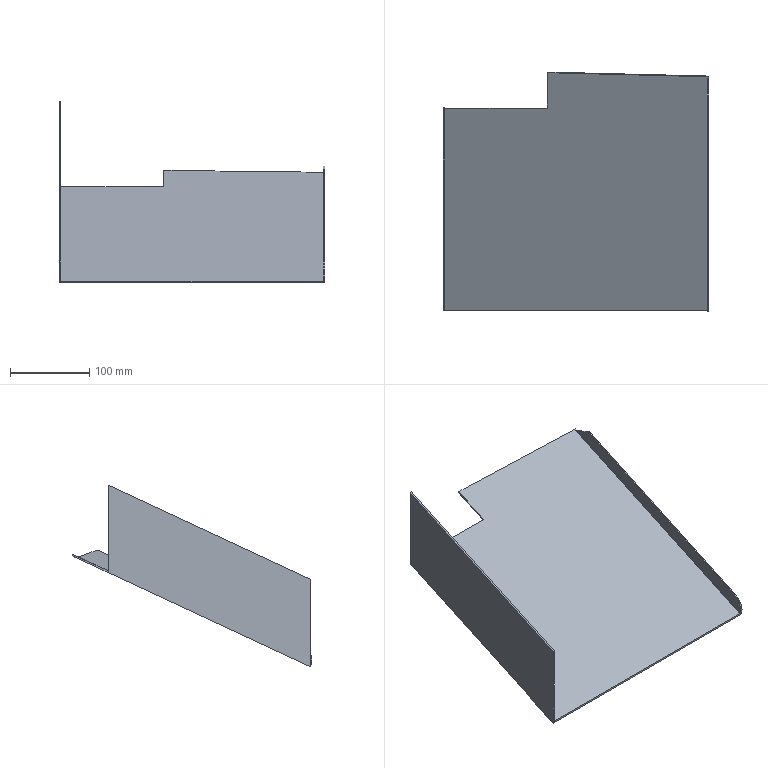Part | NX | features solid 2 | 1 solid | 15 faces | box 335 x 302.219 x 229.246 mm | volume 273833 mm3 | plane 13 | spline 1 | cylinder 1 | commonest cylinder face diameters 40 x1
STEP:
#1=CARTESIAN_POINT('',(-607.,-820.,-270.764));
#2=VERTEX_POINT('',#1);
#3=CARTESIAN_POINT('',(-938.,-820.,-270.764));
#4=VERTEX_POINT('',#3);
#5=CARTESIAN_POINT('',(1065.,-820.,-270.764));
#6=DIRECTION('',(1.,0.,0.));
#7=VECTOR('',#6,1000.);
#8=LINE('',#5,#7);
#9=EDGE_CURVE('',#2,#4,#8,.F.);
#10=ORIENTED_EDGE('',*,*,#9,.T.);
#11=CARTESIAN_POINT('',(-938.,-820.,-162.633));
#12=VERTEX_POINT('',#11);
#13=CARTESIAN_POINT('',(-938.,-820.,-730.));
#14=DIRECTION('',(0.,0.,1.));
#15=VECTOR('',#14,1000.);
#16=LINE('',#13,#15);
#17=EDGE_CURVE('',#12,#4,#16,.F.);
#18=ORIENTED_EDGE('',*,*,#17,.F.);
#19=CARTESIAN_POINT('',(-940.,-820.,-162.633));
#20=VERTEX_POINT('',#19);
#21=CARTESIAN_POINT('',(-940.,-820.,-162.633));
#22=DIRECTION('',(1.,0.,0.));
#23=VECTOR('',#22,1000.);
#24=LINE('',#21,#23);
#25=EDGE_CURVE('',#20,#12,#24,.T.);
#26=ORIENTED_EDGE('',*,*,#25,.F.);
#27=CARTESIAN_POINT('',(-940.,-820.,-272.971));
#28=VERTEX_POINT('',#27);
#29=CARTESIAN_POINT('',(-940.,-820.,-151.933));
#30=DIRECTION('',(0.,0.,1.));
#31=VECTOR('',#30,1000.);
#32=LINE('',#29,#31);
#33=EDGE_CURVE('',#28,#20,#32,.T.);
#34=ORIENTED_EDGE('',*,*,#33,.F.);
#35=CARTESIAN_POINT('',(-607.,-820.,-272.971));
#36=VERTEX_POINT('',#35);
#37=CARTESIAN_POINT('',(1065.,-820.,-272.971));
#38=DIRECTION('',(1.,0.,0.));
#39=VECTOR('',#38,1000.);
#40=LINE('',#37,#39);
#41=EDGE_CURVE('',#36,#28,#40,.F.);
#42=ORIENTED_EDGE('',*,*,#41,.F.);
#43=CARTESIAN_POINT('',(-607.,-820.,-730.));
#44=DIRECTION('',(0.,0.,1.));
#45=VECTOR('',#44,1000.);
#46=LINE('',#43,#45);
#47=EDGE_CURVE('',#2,#36,#46,.F.);
#48=ORIENTED_EDGE('',*,*,#47,.F.);
#49=EDGE_LOOP('',(#10,#18,#26,#34,#42,#48));
#50=FACE_BOUND('',#49,.T.);
#51=CARTESIAN_POINT('',(1065.,-820.,-730.));
#52=DIRECTION('',(0.,1.,0.));
#53=DIRECTION('',(-1.,0.,0.));
#54=AXIS2_PLACEMENT_3D('',#51,#52,#53);
#55=PLANE('',#54);
#56=ADVANCED_FACE('',(#50),#55,.F.);
#57=CARTESIAN_POINT('',(-808.587,-565.,-151.855));
#58=VERTEX_POINT('',#57);
#59=CARTESIAN_POINT('',(-938.,-565.,-151.855));
#60=VERTEX_POINT('',#59);
#61=CARTESIAN_POINT('',(-888.494,-565.,-151.855));
#62=DIRECTION('',(1.,0.,0.));
#63=VECTOR('',#62,1000.);
#64=LINE('',#61,#63);
#65=EDGE_CURVE('',#58,#60,#64,.F.);
#66=ORIENTED_EDGE('',*,*,#65,.T.);
#67=CARTESIAN_POINT('',(-938.,-565.167,-151.933));
#68=DIRECTION('',(0.,-0.9063,-0.4226));
#69=VECTOR('',#68,1000.);
#70=LINE('',#67,#69);
#71=EDGE_CURVE('',#60,#4,#70,.T.);
#72=ORIENTED_EDGE('',*,*,#71,.T.);
#73=ORIENTED_EDGE('',*,*,#9,.F.);
#74=CARTESIAN_POINT('',(-607.,-527.391,-134.318));
#75=VERTEX_POINT('',#74);
#76=CARTESIAN_POINT('',(-607.,-565.167,-151.933));
#77=DIRECTION('',(0.,-0.9063,-0.4226));
#78=VECTOR('',#77,1000.);
#79=LINE('',#76,#78);
#80=EDGE_CURVE('',#75,#2,#79,.T.);
#81=ORIENTED_EDGE('',*,*,#80,.F.);
#82=CARTESIAN_POINT('',(-605.,-527.391,-134.318));
#83=VERTEX_POINT('',#82);
#84=CARTESIAN_POINT('',(-808.587,-527.391,-134.318));
#85=DIRECTION('',(1.,0.,0.));
#86=VECTOR('',#85,1000.);
#87=LINE('',#84,#86);
#88=EDGE_CURVE('',#83,#75,#87,.F.);
#89=ORIENTED_EDGE('',*,*,#88,.F.);
#90=CARTESIAN_POINT('',(-605.,-525.579,-133.473));
#91=VERTEX_POINT('',#90);
#92=CARTESIAN_POINT('',(-605.,-656.469,-194.508));
#93=DIRECTION('',(0.,-0.9063,-0.4226));
#94=VECTOR('',#93,1000.);
#95=LINE('',#92,#94);
#96=EDGE_CURVE('',#91,#83,#95,.T.);
#97=ORIENTED_EDGE('',*,*,#96,.F.);
#98=CARTESIAN_POINT('',(-793.598,-520.901,-131.292));
#99=VERTEX_POINT('',#98);
#100=CARTESIAN_POINT('',(-605.,-525.579,-133.473));
#101=CARTESIAN_POINT('',(-670.132,-524.081,-132.774));
#102=CARTESIAN_POINT('',(-732.998,-522.521,-132.047));
#103=CARTESIAN_POINT('',(-793.598,-520.901,-131.292));
#104=B_SPLINE_CURVE_WITH_KNOTS('',3,(#100,#101,#102,#103),.UNSPECIFIED.,.F.,.F.,(4,4),(0.,1.),.UNSPECIFIED.);
#105=EDGE_CURVE('',#91,#99,#104,.T.);
#106=ORIENTED_EDGE('',*,*,#105,.T.);
#107=CARTESIAN_POINT('',(-808.599,-520.5,-131.104));
#108=VERTEX_POINT('',#107);
#109=CARTESIAN_POINT('',(-793.598,-520.901,-131.292));
#110=CARTESIAN_POINT('',(-798.598,-520.767,-131.229));
#111=CARTESIAN_POINT('',(-803.598,-520.633,-131.167));
#112=CARTESIAN_POINT('',(-808.599,-520.5,-131.104));
#113=B_SPLINE_CURVE_WITH_KNOTS('',3,(#109,#110,#111,#112),.UNSPECIFIED.,.F.,.F.,(4,4),(0.,1.),.UNSPECIFIED.);
#114=EDGE_CURVE('',#108,#99,#113,.F.);
#115=ORIENTED_EDGE('',*,*,#114,.F.);
#116=CARTESIAN_POINT('',(-808.599,-520.5,-131.104));
#117=CARTESIAN_POINT('',(-808.595,-535.333,-138.021));
#118=CARTESIAN_POINT('',(-808.591,-550.167,-144.938));
#119=CARTESIAN_POINT('',(-808.587,-565.,-151.855));
#120=B_SPLINE_CURVE_WITH_KNOTS('',3,(#116,#117,#118,#119),.UNSPECIFIED.,.F.,.F.,(4,4),(0.,0.9814),.UNSPECIFIED.);
#121=EDGE_CURVE('',#58,#108,#120,.F.);
#122=ORIENTED_EDGE('',*,*,#121,.F.);
#123=EDGE_LOOP('',(#66,#72,#73,#81,#89,#97,#106,#115,#122));
#124=FACE_BOUND('',#123,.T.);
#125=CARTESIAN_POINT('',(-808.587,-565.167,-151.933));
#126=DIRECTION('',(0.,-0.4226,0.9063));
#127=DIRECTION('',(1.,0.,0.));
#128=AXIS2_PLACEMENT_3D('',#125,#126,#127);
#129=PLANE('',#128);
#130=ADVANCED_FACE('',(#124),#129,.T.);
#131=ORIENTED_EDGE('',*,*,#96,.T.);
#132=CARTESIAN_POINT('',(-605.,-551.312,-125.612));
#133=VERTEX_POINT('',#132);
#134=CARTESIAN_POINT('',(-605.,-551.312,-125.612));
#135=DIRECTION('',(0.,0.9397,-0.342));
#136=VECTOR('',#135,1000.);
#137=LINE('',#134,#136);
#138=EDGE_CURVE('',#83,#133,#137,.F.);
#139=ORIENTED_EDGE('',*,*,#138,.T.);
#140=CARTESIAN_POINT('',(-605.,-810.326,-246.392));
#141=VERTEX_POINT('',#140);
#142=CARTESIAN_POINT('',(-605.,-533.186,-117.159));
#143=DIRECTION('',(0.,-0.9063,-0.4226));
#144=VECTOR('',#143,1000.);
#145=LINE('',#142,#144);
#146=EDGE_CURVE('',#133,#141,#145,.T.);
#147=ORIENTED_EDGE('',*,*,#146,.T.);
#148=CARTESIAN_POINT('',(-605.,-820.,-272.971));
#149=VERTEX_POINT('',#148);
#150=CARTESIAN_POINT('',(-605.,-801.874,-264.518));
#151=DIRECTION('',(-1.,0.,0.));
#152=DIRECTION('',(0.,0.,1.));
#153=AXIS2_PLACEMENT_3D('',#150,#151,#152);
#154=CIRCLE('',#153,20.);
#155=EDGE_CURVE('',#141,#149,#154,.F.);
#156=ORIENTED_EDGE('',*,*,#155,.T.);
#157=CARTESIAN_POINT('',(-605.,-524.733,-135.285));
#158=VERTEX_POINT('',#157);
#159=CARTESIAN_POINT('',(-605.,-655.624,-196.321));
#160=DIRECTION('',(0.,-0.9063,-0.4226));
#161=VECTOR('',#160,1000.);
#162=LINE('',#159,#161);
#163=EDGE_CURVE('',#158,#149,#162,.T.);
#164=ORIENTED_EDGE('',*,*,#163,.F.);
#165=CARTESIAN_POINT('',(-605.,-524.733,-135.285));
#166=CARTESIAN_POINT('',(-605.,-525.015,-134.681));
#167=CARTESIAN_POINT('',(-605.,-525.297,-134.077));
#168=CARTESIAN_POINT('',(-605.,-525.579,-133.473));
#169=B_SPLINE_CURVE_WITH_KNOTS('',3,(#165,#166,#167,#168),.UNSPECIFIED.,.F.,.F.,(4,4),(0.,1.),.UNSPECIFIED.);
#170=EDGE_CURVE('',#91,#158,#169,.F.);
#171=ORIENTED_EDGE('',*,*,#170,.F.);
#172=EDGE_LOOP('',(#131,#139,#147,#156,#164,#171));
#173=FACE_BOUND('',#172,.T.);
#174=CARTESIAN_POINT('',(-605.,-656.469,-194.508));
#175=DIRECTION('',(1.,0.,0.));
#176=DIRECTION('',(0.,0.,-1.));
#177=AXIS2_PLACEMENT_3D('',#174,#175,#176);
#178=PLANE('',#177);
#179=ADVANCED_FACE('',(#173),#178,.T.);
#180=CARTESIAN_POINT('',(-793.598,-520.055,-133.104));
#181=VERTEX_POINT('',#180);
#182=CARTESIAN_POINT('',(-605.,-524.733,-135.285));
#183=CARTESIAN_POINT('',(-670.132,-523.235,-134.587));
#184=CARTESIAN_POINT('',(-732.998,-521.676,-133.86));
#185=CARTESIAN_POINT('',(-793.598,-520.055,-133.104));
#186=B_SPLINE_CURVE_WITH_KNOTS('',3,(#182,#183,#184,#185),.UNSPECIFIED.,.F.,.F.,(4,4),(0.,1.),.UNSPECIFIED.);
#187=EDGE_CURVE('',#158,#181,#186,.T.);
#188=ORIENTED_EDGE('',*,*,#187,.T.);
#189=CARTESIAN_POINT('',(-793.598,-520.901,-131.292));
#190=CARTESIAN_POINT('',(-793.598,-520.619,-131.896));
#191=CARTESIAN_POINT('',(-793.598,-520.337,-132.5));
#192=CARTESIAN_POINT('',(-793.598,-520.055,-133.104));
#193=B_SPLINE_CURVE_WITH_KNOTS('',3,(#189,#190,#191,#192),.UNSPECIFIED.,.F.,.F.,(4,4),(0.,1.),.UNSPECIFIED.);
#194=EDGE_CURVE('',#99,#181,#193,.T.);
#195=ORIENTED_EDGE('',*,*,#194,.F.);
#196=ORIENTED_EDGE('',*,*,#105,.F.);
#197=ORIENTED_EDGE('',*,*,#170,.T.);
#198=EDGE_LOOP('',(#188,#195,#196,#197));
#199=FACE_BOUND('',#198,.T.);
#200=CARTESIAN_POINT('',(-605.,-525.579,-133.473));
#201=CARTESIAN_POINT('',(-605.,-524.733,-135.285));
#202=CARTESIAN_POINT('',(-670.132,-524.081,-132.774));
#203=CARTESIAN_POINT('',(-670.132,-523.235,-134.587));
#204=CARTESIAN_POINT('',(-732.998,-522.521,-132.047));
#205=CARTESIAN_POINT('',(-732.998,-521.676,-133.86));
#206=CARTESIAN_POINT('',(-793.598,-520.901,-131.292));
#207=CARTESIAN_POINT('',(-793.598,-520.055,-133.104));
#208=B_SPLINE_SURFACE_WITH_KNOTS('',3,1,((#200,#201),(#202,#203),(#204,#205),(#206,#207)),.SURF_OF_LINEAR_EXTRUSION.,.F.,.F.,.F.,(4,4),(2,2),(0.,1.),(0.,1.),.PIECEWISE_BEZIER_KNOTS.);
#209=ADVANCED_FACE('',(#199),#208,.F.);
#210=CARTESIAN_POINT('',(-808.599,-519.654,-132.917));
#211=VERTEX_POINT('',#210);
#212=CARTESIAN_POINT('',(-793.598,-520.055,-133.104));
#213=CARTESIAN_POINT('',(-798.598,-519.922,-133.042));
#214=CARTESIAN_POINT('',(-803.598,-519.788,-132.979));
#215=CARTESIAN_POINT('',(-808.599,-519.654,-132.917));
#216=B_SPLINE_CURVE_WITH_KNOTS('',3,(#212,#213,#214,#215),.UNSPECIFIED.,.F.,.F.,(4,4),(0.,1.),.UNSPECIFIED.);
#217=EDGE_CURVE('',#211,#181,#216,.F.);
#218=ORIENTED_EDGE('',*,*,#217,.F.);
#219=CARTESIAN_POINT('',(-808.599,-519.654,-132.917));
#220=CARTESIAN_POINT('',(-808.599,-519.936,-132.313));
#221=CARTESIAN_POINT('',(-808.599,-520.218,-131.709));
#222=CARTESIAN_POINT('',(-808.599,-520.5,-131.104));
#223=B_SPLINE_CURVE_WITH_KNOTS('',3,(#219,#220,#221,#222),.UNSPECIFIED.,.F.,.F.,(4,4),(0.,1.),.UNSPECIFIED.);
#224=EDGE_CURVE('',#108,#211,#223,.F.);
#225=ORIENTED_EDGE('',*,*,#224,.F.);
#226=ORIENTED_EDGE('',*,*,#114,.T.);
#227=ORIENTED_EDGE('',*,*,#194,.T.);
#228=EDGE_LOOP('',(#218,#225,#226,#227));
#229=FACE_BOUND('',#228,.T.);
#230=CARTESIAN_POINT('',(-793.598,-520.901,-131.292));
#231=DIRECTION('',(0.02949,0.9059,0.4224));
#232=DIRECTION('',(0.,-0.4226,0.9063));
#233=AXIS2_PLACEMENT_3D('',#230,#231,#232);
#234=PLANE('',#233);
#235=ADVANCED_FACE('',(#229),#234,.T.);
#236=CARTESIAN_POINT('',(-808.587,-565.,-154.062));
#237=VERTEX_POINT('',#236);
#238=CARTESIAN_POINT('',(-808.599,-519.654,-132.917));
#239=CARTESIAN_POINT('',(-808.595,-534.77,-139.965));
#240=CARTESIAN_POINT('',(-808.591,-549.885,-147.014));
#241=CARTESIAN_POINT('',(-808.587,-565.,-154.062));
#242=B_SPLINE_CURVE_WITH_KNOTS('',3,(#238,#239,#240,#241),.UNSPECIFIED.,.F.,.F.,(4,4),(0.,1.),.UNSPECIFIED.);
#243=EDGE_CURVE('',#237,#211,#242,.F.);
#244=ORIENTED_EDGE('',*,*,#243,.F.);
#245=CARTESIAN_POINT('',(-808.6,-565.,-17.313));
#246=DIRECTION('',(-0.00009751,0.,1.));
#247=VECTOR('',#246,1000.);
#248=LINE('',#245,#247);
#249=EDGE_CURVE('',#58,#237,#248,.F.);
#250=ORIENTED_EDGE('',*,*,#249,.F.);
#251=ORIENTED_EDGE('',*,*,#121,.T.);
#252=ORIENTED_EDGE('',*,*,#224,.T.);
#253=EDGE_LOOP('',(#244,#250,#251,#252));
#254=FACE_BOUND('',#253,.T.);
#255=CARTESIAN_POINT('',(-808.599,-520.5,-131.104));
#256=DIRECTION('',(-1.,-0.0002091,-0.00009751));
#257=DIRECTION('',(0.0002091,-1.,0.));
#258=AXIS2_PLACEMENT_3D('',#255,#256,#257);
#259=PLANE('',#258);
#260=ADVANCED_FACE('',(#254),#259,.T.);
#261=CARTESIAN_POINT('',(-940.,-565.,-154.062));
#262=VERTEX_POINT('',#261);
#263=CARTESIAN_POINT('',(-888.494,-565.,-154.062));
#264=DIRECTION('',(1.,0.,0.));
#265=VECTOR('',#264,1000.);
#266=LINE('',#263,#265);
#267=EDGE_CURVE('',#237,#262,#266,.F.);
#268=ORIENTED_EDGE('',*,*,#267,.T.);
#269=CARTESIAN_POINT('',(-940.,-565.,-43.724));
#270=VERTEX_POINT('',#269);
#271=CARTESIAN_POINT('',(-940.,-565.,-151.933));
#272=DIRECTION('',(0.,0.,1.));
#273=VECTOR('',#272,1000.);
#274=LINE('',#271,#273);
#275=EDGE_CURVE('',#270,#262,#274,.F.);
#276=ORIENTED_EDGE('',*,*,#275,.F.);
#277=CARTESIAN_POINT('',(-938.,-565.,-43.724));
#278=VERTEX_POINT('',#277);
#279=CARTESIAN_POINT('',(-888.494,-565.,-43.724));
#280=DIRECTION('',(-1.,0.,0.));
#281=VECTOR('',#280,1000.);
#282=LINE('',#279,#281);
#283=EDGE_CURVE('',#278,#270,#282,.T.);
#284=ORIENTED_EDGE('',*,*,#283,.F.);
#285=CARTESIAN_POINT('',(-938.,-565.,-154.062));
#286=DIRECTION('',(0.,0.,-1.));
#287=VECTOR('',#286,1000.);
#288=LINE('',#285,#287);
#289=EDGE_CURVE('',#60,#278,#288,.F.);
#290=ORIENTED_EDGE('',*,*,#289,.F.);
#291=ORIENTED_EDGE('',*,*,#65,.F.);
#292=ORIENTED_EDGE('',*,*,#249,.T.);
#293=EDGE_LOOP('',(#268,#276,#284,#290,#291,#292));
#294=FACE_BOUND('',#293,.T.);
#295=CARTESIAN_POINT('',(-888.494,-565.,-17.321));
#296=DIRECTION('',(0.,1.,0.));
#297=DIRECTION('',(-1.,0.,0.));
#298=AXIS2_PLACEMENT_3D('',#295,#296,#297);
#299=PLANE('',#298);
#300=ADVANCED_FACE('',(#294),#299,.T.);
#301=ORIENTED_EDGE('',*,*,#275,.T.);
#302=CARTESIAN_POINT('',(-940.,-564.322,-153.746));
#303=DIRECTION('',(0.,-0.9063,-0.4226));
#304=VECTOR('',#303,1000.);
#305=LINE('',#302,#304);
#306=EDGE_CURVE('',#262,#28,#305,.T.);
#307=ORIENTED_EDGE('',*,*,#306,.T.);
#308=ORIENTED_EDGE('',*,*,#33,.T.);
#309=CARTESIAN_POINT('',(-940.,-606.583,-63.115));
#310=DIRECTION('',(0.,0.9063,0.4226));
#311=VECTOR('',#310,1000.);
#312=LINE('',#309,#311);
#313=EDGE_CURVE('',#270,#20,#312,.F.);
#314=ORIENTED_EDGE('',*,*,#313,.F.);
#315=EDGE_LOOP('',(#301,#307,#308,#314));
#316=FACE_BOUND('',#315,.T.);
#317=CARTESIAN_POINT('',(-940.,-565.167,-151.933));
#318=DIRECTION('',(1.,0.,0.));
#319=DIRECTION('',(0.,0.,-1.));
#320=AXIS2_PLACEMENT_3D('',#317,#318,#319);
#321=PLANE('',#320);
#322=ADVANCED_FACE('',(#316),#321,.F.);
#323=ORIENTED_EDGE('',*,*,#306,.F.);
#324=ORIENTED_EDGE('',*,*,#267,.F.);
#325=ORIENTED_EDGE('',*,*,#243,.T.);
#326=ORIENTED_EDGE('',*,*,#217,.T.);
#327=ORIENTED_EDGE('',*,*,#187,.F.);
#328=ORIENTED_EDGE('',*,*,#163,.T.);
#329=CARTESIAN_POINT('',(1065.,-820.,-272.971));
#330=DIRECTION('',(1.,0.,0.));
#331=VECTOR('',#330,1000.);
#332=LINE('',#329,#331);
#333=EDGE_CURVE('',#149,#36,#332,.F.);
#334=ORIENTED_EDGE('',*,*,#333,.T.);
#335=ORIENTED_EDGE('',*,*,#41,.T.);
#336=EDGE_LOOP('',(#323,#324,#325,#326,#327,#328,#334,#335));
#337=FACE_BOUND('',#336,.T.);
#338=CARTESIAN_POINT('',(-808.587,-564.322,-153.746));
#339=DIRECTION('',(0.,-0.4226,0.9063));
#340=DIRECTION('',(1.,0.,0.));
#341=AXIS2_PLACEMENT_3D('',#338,#339,#340);
#342=PLANE('',#341);
#343=ADVANCED_FACE('',(#337),#342,.F.);
#344=ORIENTED_EDGE('',*,*,#146,.F.);
#345=CARTESIAN_POINT('',(-607.,-551.312,-125.612));
#346=VERTEX_POINT('',#345);
#347=CARTESIAN_POINT('',(-605.,-551.312,-125.612));
#348=DIRECTION('',(-1.,0.,0.));
#349=VECTOR('',#348,1000.);
#350=LINE('',#347,#349);
#351=EDGE_CURVE('',#133,#346,#350,.T.);
#352=ORIENTED_EDGE('',*,*,#351,.T.);
#353=CARTESIAN_POINT('',(-607.,-810.326,-246.392));
#354=VERTEX_POINT('',#353);
#355=CARTESIAN_POINT('',(-607.,-533.186,-117.159));
#356=DIRECTION('',(0.,-0.9063,-0.4226));
#357=VECTOR('',#356,1000.);
#358=LINE('',#355,#357);
#359=EDGE_CURVE('',#346,#354,#358,.T.);
#360=ORIENTED_EDGE('',*,*,#359,.T.);
#361=CARTESIAN_POINT('',(-605.,-810.326,-246.392));
#362=DIRECTION('',(1.,0.,0.));
#363=VECTOR('',#362,1000.);
#364=LINE('',#361,#363);
#365=EDGE_CURVE('',#354,#141,#364,.T.);
#366=ORIENTED_EDGE('',*,*,#365,.T.);
#367=EDGE_LOOP('',(#344,#352,#360,#366));
#368=FACE_BOUND('',#367,.T.);
#369=CARTESIAN_POINT('',(-605.,-533.186,-117.159));
#370=DIRECTION('',(0.,0.4226,-0.9063));
#371=DIRECTION('',(0.,-0.9063,-0.4226));
#372=AXIS2_PLACEMENT_3D('',#369,#370,#371);
#373=PLANE('',#372);
#374=ADVANCED_FACE('',(#368),#373,.F.);
#375=ORIENTED_EDGE('',*,*,#80,.T.);
#376=ORIENTED_EDGE('',*,*,#47,.T.);
#377=CARTESIAN_POINT('',(-607.,-801.874,-264.518));
#378=DIRECTION('',(-1.,0.,0.));
#379=DIRECTION('',(0.,0.,1.));
#380=AXIS2_PLACEMENT_3D('',#377,#378,#379);
#381=CIRCLE('',#380,20.);
#382=EDGE_CURVE('',#36,#354,#381,.T.);
#383=ORIENTED_EDGE('',*,*,#382,.T.);
#384=ORIENTED_EDGE('',*,*,#359,.F.);
#385=CARTESIAN_POINT('',(-607.,-524.733,-135.285));
#386=DIRECTION('',(0.,-0.9397,0.342));
#387=VECTOR('',#386,1000.);
#388=LINE('',#385,#387);
#389=EDGE_CURVE('',#346,#75,#388,.F.);
#390=ORIENTED_EDGE('',*,*,#389,.T.);
#391=EDGE_LOOP('',(#375,#376,#383,#384,#390));
#392=FACE_BOUND('',#391,.T.);
#393=CARTESIAN_POINT('',(-607.,-524.733,-135.285));
#394=DIRECTION('',(-1.,0.,0.));
#395=DIRECTION('',(0.,0.,1.));
#396=AXIS2_PLACEMENT_3D('',#393,#394,#395);
#397=PLANE('',#396);
#398=ADVANCED_FACE('',(#392),#397,.T.);
#399=ORIENTED_EDGE('',*,*,#155,.F.);
#400=ORIENTED_EDGE('',*,*,#365,.F.);
#401=ORIENTED_EDGE('',*,*,#382,.F.);
#402=ORIENTED_EDGE('',*,*,#333,.F.);
#403=EDGE_LOOP('',(#399,#400,#401,#402));
#404=FACE_BOUND('',#403,.T.);
#405=CARTESIAN_POINT('',(-605.,-801.874,-264.518));
#406=DIRECTION('',(1.,0.,0.));
#407=DIRECTION('',(0.,0.,-1.));
#408=AXIS2_PLACEMENT_3D('',#405,#406,#407);
#409=CYLINDRICAL_SURFACE('',#408,20.);
#410=ADVANCED_FACE('',(#404),#409,.T.);
#411=ORIENTED_EDGE('',*,*,#138,.F.);
#412=ORIENTED_EDGE('',*,*,#88,.T.);
#413=ORIENTED_EDGE('',*,*,#389,.F.);
#414=ORIENTED_EDGE('',*,*,#351,.F.);
#415=EDGE_LOOP('',(#411,#412,#413,#414));
#416=FACE_BOUND('',#415,.T.);
#417=CARTESIAN_POINT('',(-605.,-551.312,-125.612));
#418=DIRECTION('',(0.,-0.342,-0.9397));
#419=DIRECTION('',(0.,0.9397,-0.342));
#420=AXIS2_PLACEMENT_3D('',#417,#418,#419);
#421=PLANE('',#420);
#422=ADVANCED_FACE('',(#416),#421,.F.);
#423=CARTESIAN_POINT('',(-938.,-607.262,-63.431));
#424=DIRECTION('',(0.,0.9063,0.4226));
#425=VECTOR('',#424,1000.);
#426=LINE('',#423,#425);
#427=EDGE_CURVE('',#278,#12,#426,.F.);
#428=ORIENTED_EDGE('',*,*,#427,.F.);
#429=ORIENTED_EDGE('',*,*,#283,.T.);
#430=ORIENTED_EDGE('',*,*,#313,.T.);
#431=ORIENTED_EDGE('',*,*,#25,.T.);
#432=EDGE_LOOP('',(#428,#429,#430,#431));
#433=FACE_BOUND('',#432,.T.);
#434=CARTESIAN_POINT('',(-940.,-607.262,-63.431));
#435=DIRECTION('',(0.,0.4226,-0.9063));
#436=DIRECTION('',(0.,-0.9063,-0.4226));
#437=AXIS2_PLACEMENT_3D('',#434,#435,#436);
#438=PLANE('',#437);
#439=ADVANCED_FACE('',(#433),#438,.F.);
#440=ORIENTED_EDGE('',*,*,#17,.T.);
#441=ORIENTED_EDGE('',*,*,#71,.F.);
#442=ORIENTED_EDGE('',*,*,#289,.T.);
#443=ORIENTED_EDGE('',*,*,#427,.T.);
#444=EDGE_LOOP('',(#440,#441,#442,#443));
#445=FACE_BOUND('',#444,.T.);
#446=CARTESIAN_POINT('',(-938.,-565.,-154.062));
#447=DIRECTION('',(-1.,0.,0.));
#448=DIRECTION('',(0.,0.,1.));
#449=AXIS2_PLACEMENT_3D('',#446,#447,#448);
#450=PLANE('',#449);
#451=ADVANCED_FACE('',(#445),#450,.F.);
#452=CLOSED_SHELL('',(#56,#130,#179,#209,#235,#260,#300,#322,#343,#374,#398,#410,#422,#439,#451));
#453=MANIFOLD_SOLID_BREP('',#452);
#454=(LENGTH_UNIT()NAMED_UNIT(*)SI_UNIT(.MILLI.,.METRE.));
#455=UNCERTAINTY_MEASURE_WITH_UNIT(LENGTH_MEASURE(0.0508),#454,'','');
#456=(NAMED_UNIT(*)PLANE_ANGLE_UNIT()SI_UNIT($,.RADIAN.));
#457=(NAMED_UNIT(*)SI_UNIT($,.STERADIAN.)SOLID_ANGLE_UNIT());
#458=(GEOMETRIC_REPRESENTATION_CONTEXT(3)GLOBAL_UNCERTAINTY_ASSIGNED_CONTEXT((#455))GLOBAL_UNIT_ASSIGNED_CONTEXT((#454,#456,#457))REPRESENTATION_CONTEXT('',''));
#459=ADVANCED_BREP_SHAPE_REPRESENTATION('',(#453),#458);